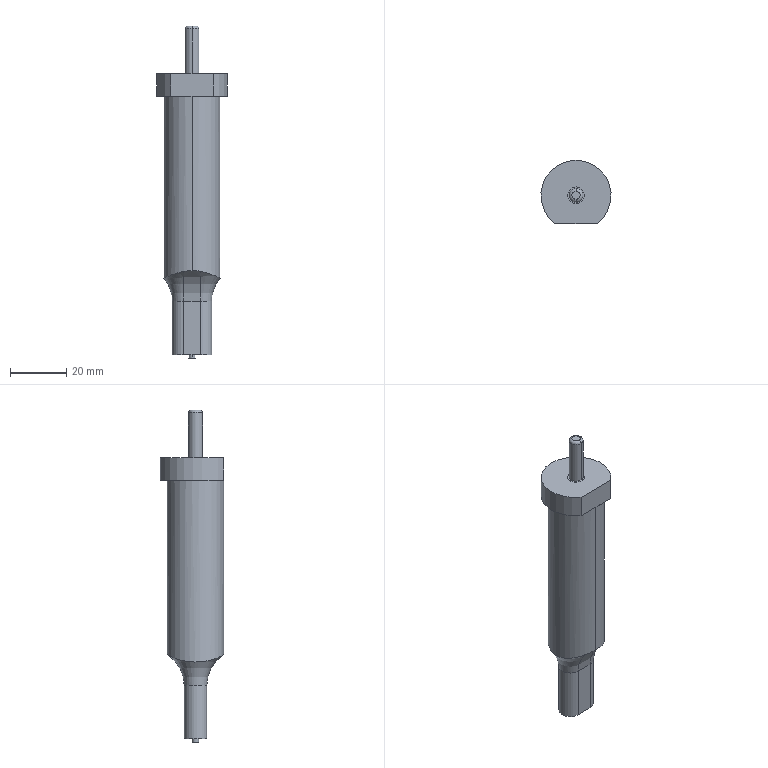Part | STEP file | 1_id3642_x_t | 1 solid | 27 faces | box 25 x 22.5 x 118.2 mm | volume 27347 mm3 | cylinder 14 | plane 9 | torus 4 | commonest cylinder face diameters 2.26 x2 5 x2 6 x2 8.05 x2 20 x2 25 x2
STEP:
#1=CARTESIAN_POINT('',(3587.234,-220.45,22.438));
#2=VERTEX_POINT('',#1);
#3=CARTESIAN_POINT('',(3587.234,-220.45,84.5));
#4=VERTEX_POINT('',#3);
#5=CARTESIAN_POINT('',(3587.234,-220.45,38.5));
#6=DIRECTION('',(0.,0.,1.));
#7=VECTOR('',#6,1.);
#8=LINE('',#5,#7);
#9=EDGE_CURVE('',#2,#4,#8,.T.);
#10=ORIENTED_EDGE('',*,*,#9,.F.);
#11=CARTESIAN_POINT('',(3584.234,-220.911,22.129));
#12=VERTEX_POINT('',#11);
#13=CARTESIAN_POINT('',(3587.234,-220.45,22.438));
#14=CARTESIAN_POINT('',(3586.2,-220.45,22.438));
#15=CARTESIAN_POINT('',(3585.2,-220.607,22.342));
#16=CARTESIAN_POINT('',(3584.234,-220.911,22.129));
#17=B_SPLINE_CURVE_WITH_KNOTS('',3,(#13,#14,#15,#16),.UNSPECIFIED.,.F.,.F.,(4,4),(0.,1.),.UNSPECIFIED.);
#18=EDGE_CURVE('',#2,#12,#17,.T.);
#19=ORIENTED_EDGE('',*,*,#18,.T.);
#20=CARTESIAN_POINT('',(3584.234,-239.989,22.129));
#21=VERTEX_POINT('',#20);
#22=CARTESIAN_POINT('',(3584.234,-220.911,22.129));
#23=CARTESIAN_POINT('',(3582.209,-221.547,21.68));
#24=CARTESIAN_POINT('',(3580.455,-222.805,21.143));
#25=CARTESIAN_POINT('',(3577.956,-226.171,20.175));
#26=CARTESIAN_POINT('',(3577.238,-228.29,19.779));
#27=CARTESIAN_POINT('',(3577.23,-232.57,19.774));
#28=CARTESIAN_POINT('',(3577.946,-234.707,20.17));
#29=CARTESIAN_POINT('',(3580.438,-238.079,21.137));
#30=CARTESIAN_POINT('',(3582.208,-239.352,21.68));
#31=CARTESIAN_POINT('',(3584.234,-239.989,22.129));
#32=B_SPLINE_CURVE_WITH_KNOTS('',3,(#22,#23,#24,#25,#26,#27,#28,#29,#30,#31),.UNSPECIFIED.,.F.,.F.,(4,2,2,2,4),(0.,0.25,0.5,0.75,1.),.UNSPECIFIED.);
#33=EDGE_CURVE('',#12,#21,#32,.T.);
#34=ORIENTED_EDGE('',*,*,#33,.T.);
#35=CARTESIAN_POINT('',(3587.234,-240.45,22.438));
#36=VERTEX_POINT('',#35);
#37=CARTESIAN_POINT('',(3584.234,-239.989,22.129));
#38=CARTESIAN_POINT('',(3585.2,-240.293,22.342));
#39=CARTESIAN_POINT('',(3586.2,-240.45,22.438));
#40=CARTESIAN_POINT('',(3587.234,-240.45,22.438));
#41=B_SPLINE_CURVE_WITH_KNOTS('',3,(#37,#38,#39,#40),.UNSPECIFIED.,.F.,.F.,(4,4),(0.,1.),.UNSPECIFIED.);
#42=EDGE_CURVE('',#21,#36,#41,.T.);
#43=ORIENTED_EDGE('',*,*,#42,.T.);
#44=CARTESIAN_POINT('',(3587.234,-240.45,84.5));
#45=VERTEX_POINT('',#44);
#46=CARTESIAN_POINT('',(3587.234,-240.45,38.5));
#47=DIRECTION('',(0.,0.,-1.));
#48=VECTOR('',#47,1.);
#49=LINE('',#46,#48);
#50=EDGE_CURVE('',#45,#36,#49,.T.);
#51=ORIENTED_EDGE('',*,*,#50,.F.);
#52=CARTESIAN_POINT('',(3587.234,-230.45,84.5));
#53=DIRECTION('',(0.,0.,1.));
#54=DIRECTION('',(0.,1.,0.));
#55=AXIS2_PLACEMENT_3D('',#52,#53,#54);
#56=CIRCLE('',#55,10.);
#57=EDGE_CURVE('',#4,#45,#56,.T.);
#58=ORIENTED_EDGE('',*,*,#57,.F.);
#59=EDGE_LOOP('',(#10,#19,#34,#43,#51,#58));
#60=FACE_OUTER_BOUND('',#59,.T.);
#61=CARTESIAN_POINT('',(3587.234,-230.45,38.5));
#62=DIRECTION('',(0.,0.,-1.));
#63=DIRECTION('',(0.,-1.,0.));
#64=AXIS2_PLACEMENT_3D('',#61,#62,#63);
#65=CYLINDRICAL_SURFACE('',#64,10.);
#66=ADVANCED_FACE('',(#60),#65,.T.);
#67=CARTESIAN_POINT('',(3587.234,-217.95,84.5));
#68=VERTEX_POINT('',#67);
#69=CARTESIAN_POINT('',(3587.234,-217.95,92.5));
#70=VERTEX_POINT('',#69);
#71=CARTESIAN_POINT('',(3587.234,-217.95,88.5));
#72=DIRECTION('',(0.,0.,1.));
#73=VECTOR('',#72,1.);
#74=LINE('',#71,#73);
#75=EDGE_CURVE('',#68,#70,#74,.T.);
#76=ORIENTED_EDGE('',*,*,#75,.F.);
#77=CARTESIAN_POINT('',(3579.734,-240.45,84.5));
#78=VERTEX_POINT('',#77);
#79=CARTESIAN_POINT('',(3587.234,-230.45,84.5));
#80=DIRECTION('',(0.,0.,1.));
#81=DIRECTION('',(0.,1.,0.));
#82=AXIS2_PLACEMENT_3D('',#79,#80,#81);
#83=CIRCLE('',#82,12.5);
#84=EDGE_CURVE('',#68,#78,#83,.T.);
#85=ORIENTED_EDGE('',*,*,#84,.T.);
#86=CARTESIAN_POINT('',(3579.734,-240.45,92.5));
#87=VERTEX_POINT('',#86);
#88=CARTESIAN_POINT('',(3579.734,-240.45,88.5));
#89=DIRECTION('',(0.,0.,1.));
#90=VECTOR('',#89,1.);
#91=LINE('',#88,#90);
#92=EDGE_CURVE('',#78,#87,#91,.T.);
#93=ORIENTED_EDGE('',*,*,#92,.T.);
#94=CARTESIAN_POINT('',(3587.234,-230.45,92.5));
#95=DIRECTION('',(0.,0.,1.));
#96=DIRECTION('',(0.,1.,0.));
#97=AXIS2_PLACEMENT_3D('',#94,#95,#96);
#98=CIRCLE('',#97,12.5);
#99=EDGE_CURVE('',#70,#87,#98,.T.);
#100=ORIENTED_EDGE('',*,*,#99,.F.);
#101=EDGE_LOOP('',(#76,#85,#93,#100));
#102=FACE_OUTER_BOUND('',#101,.T.);
#103=CARTESIAN_POINT('',(3587.234,-230.45,88.5));
#104=DIRECTION('',(0.,0.,-1.));
#105=DIRECTION('',(0.,-1.,0.));
#106=AXIS2_PLACEMENT_3D('',#103,#104,#105);
#107=CYLINDRICAL_SURFACE('',#106,12.5);
#108=ADVANCED_FACE('',(#102),#107,.T.);
#109=CARTESIAN_POINT('',(3587.234,-231.58,-7.5));
#110=VERTEX_POINT('',#109);
#111=CARTESIAN_POINT('',(3587.234,-231.58,-8.7));
#112=VERTEX_POINT('',#111);
#113=CARTESIAN_POINT('',(3587.234,-231.58,-7.5));
#114=DIRECTION('',(0.,0.,-1.));
#115=VECTOR('',#114,1.);
#116=LINE('',#113,#115);
#117=EDGE_CURVE('',#110,#112,#116,.T.);
#118=ORIENTED_EDGE('',*,*,#117,.F.);
#119=CARTESIAN_POINT('',(3587.234,-229.32,-7.5));
#120=VERTEX_POINT('',#119);
#121=CARTESIAN_POINT('',(3587.234,-230.45,-7.5));
#122=DIRECTION('',(0.,0.,1.));
#123=DIRECTION('',(0.,-1.,0.));
#124=AXIS2_PLACEMENT_3D('',#121,#122,#123);
#125=CIRCLE('',#124,1.13);
#126=EDGE_CURVE('',#120,#110,#125,.T.);
#127=ORIENTED_EDGE('',*,*,#126,.F.);
#128=CARTESIAN_POINT('',(3587.234,-229.32,-8.7));
#129=VERTEX_POINT('',#128);
#130=CARTESIAN_POINT('',(3587.234,-229.32,-7.5));
#131=DIRECTION('',(0.,0.,1.));
#132=VECTOR('',#131,1.);
#133=LINE('',#130,#132);
#134=EDGE_CURVE('',#129,#120,#133,.T.);
#135=ORIENTED_EDGE('',*,*,#134,.F.);
#136=CARTESIAN_POINT('',(3587.234,-230.45,-8.7));
#137=DIRECTION('',(0.,0.,1.));
#138=DIRECTION('',(0.,-1.,0.));
#139=AXIS2_PLACEMENT_3D('',#136,#137,#138);
#140=CIRCLE('',#139,1.13);
#141=EDGE_CURVE('',#129,#112,#140,.T.);
#142=ORIENTED_EDGE('',*,*,#141,.T.);
#143=EDGE_LOOP('',(#118,#127,#135,#142));
#144=FACE_OUTER_BOUND('',#143,.T.);
#145=CARTESIAN_POINT('',(3587.234,-230.45,-7.5));
#146=DIRECTION('',(0.,0.,1.));
#147=DIRECTION('',(0.,1.,0.));
#148=AXIS2_PLACEMENT_3D('',#145,#146,#147);
#149=CYLINDRICAL_SURFACE('',#148,1.13);
#150=ADVANCED_FACE('',(#144),#149,.T.);
#151=CARTESIAN_POINT('',(3587.234,-232.95,108.5));
#152=VERTEX_POINT('',#151);
#153=CARTESIAN_POINT('',(3587.234,-232.95,92.6));
#154=VERTEX_POINT('',#153);
#155=CARTESIAN_POINT('',(3587.234,-232.95,100.55));
#156=DIRECTION('',(0.,0.,-1.));
#157=VECTOR('',#156,1.);
#158=LINE('',#155,#157);
#159=EDGE_CURVE('',#152,#154,#158,.T.);
#160=ORIENTED_EDGE('',*,*,#159,.F.);
#161=CARTESIAN_POINT('',(3587.234,-227.95,108.5));
#162=VERTEX_POINT('',#161);
#163=CARTESIAN_POINT('',(3587.234,-230.45,108.5));
#164=DIRECTION('',(0.,0.,-1.));
#165=DIRECTION('',(0.,-1.,0.));
#166=AXIS2_PLACEMENT_3D('',#163,#164,#165);
#167=CIRCLE('',#166,2.5);
#168=EDGE_CURVE('',#152,#162,#167,.T.);
#169=ORIENTED_EDGE('',*,*,#168,.T.);
#170=CARTESIAN_POINT('',(3587.234,-227.95,92.6));
#171=VERTEX_POINT('',#170);
#172=CARTESIAN_POINT('',(3587.234,-227.95,100.55));
#173=DIRECTION('',(0.,0.,1.));
#174=VECTOR('',#173,1.);
#175=LINE('',#172,#174);
#176=EDGE_CURVE('',#171,#162,#175,.T.);
#177=ORIENTED_EDGE('',*,*,#176,.F.);
#178=CARTESIAN_POINT('',(3587.234,-230.45,92.6));
#179=DIRECTION('',(0.,0.,-1.));
#180=DIRECTION('',(0.,-1.,0.));
#181=AXIS2_PLACEMENT_3D('',#178,#179,#180);
#182=CIRCLE('',#181,2.5);
#183=EDGE_CURVE('',#154,#171,#182,.T.);
#184=ORIENTED_EDGE('',*,*,#183,.F.);
#185=EDGE_LOOP('',(#160,#169,#177,#184));
#186=FACE_OUTER_BOUND('',#185,.T.);
#187=CARTESIAN_POINT('',(3587.234,-230.45,100.55));
#188=DIRECTION('',(0.,0.,1.));
#189=DIRECTION('',(0.,1.,0.));
#190=AXIS2_PLACEMENT_3D('',#187,#188,#189);
#191=CYLINDRICAL_SURFACE('',#190,2.5);
#192=ADVANCED_FACE('',(#186),#191,.T.);
#193=CARTESIAN_POINT('',(3587.234,-228.95,109.5));
#194=VERTEX_POINT('',#193);
#195=CARTESIAN_POINT('',(3587.234,-228.95,108.5));
#196=DIRECTION('',(-1.,0.,0.));
#197=DIRECTION('',(0.,1.,0.));
#198=AXIS2_PLACEMENT_3D('',#195,#196,#197);
#199=CIRCLE('',#198,1.);
#200=EDGE_CURVE('',#194,#162,#199,.T.);
#201=ORIENTED_EDGE('',*,*,#200,.F.);
#202=CARTESIAN_POINT('',(3587.234,-231.95,109.5));
#203=VERTEX_POINT('',#202);
#204=CARTESIAN_POINT('',(3587.234,-230.45,109.5));
#205=DIRECTION('',(0.,0.,-1.));
#206=DIRECTION('',(0.,-1.,0.));
#207=AXIS2_PLACEMENT_3D('',#204,#205,#206);
#208=CIRCLE('',#207,1.5);
#209=EDGE_CURVE('',#194,#203,#208,.T.);
#210=ORIENTED_EDGE('',*,*,#209,.T.);
#211=CARTESIAN_POINT('',(3587.234,-231.95,108.5));
#212=DIRECTION('',(-1.,0.,0.));
#213=DIRECTION('',(0.,-1.,0.));
#214=AXIS2_PLACEMENT_3D('',#211,#212,#213);
#215=CIRCLE('',#214,1.);
#216=EDGE_CURVE('',#152,#203,#215,.T.);
#217=ORIENTED_EDGE('',*,*,#216,.F.);
#218=CARTESIAN_POINT('',(3587.234,-230.45,108.5));
#219=DIRECTION('',(0.,0.,-1.));
#220=DIRECTION('',(0.,-1.,0.));
#221=AXIS2_PLACEMENT_3D('',#218,#219,#220);
#222=CIRCLE('',#221,2.5);
#223=EDGE_CURVE('',#162,#152,#222,.T.);
#224=ORIENTED_EDGE('',*,*,#223,.F.);
#225=EDGE_LOOP('',(#201,#210,#217,#224));
#226=FACE_OUTER_BOUND('',#225,.T.);
#227=CARTESIAN_POINT('',(3587.234,-230.45,108.5));
#228=DIRECTION('',(0.,0.,-1.));
#229=DIRECTION('',(0.,-1.,0.));
#230=AXIS2_PLACEMENT_3D('',#227,#228,#229);
#231=TOROIDAL_SURFACE('',#230,1.5,1.);
#232=ADVANCED_FACE('',(#226),#231,.T.);
#233=CARTESIAN_POINT('',(3587.234,-233.45,92.6));
#234=VERTEX_POINT('',#233);
#235=CARTESIAN_POINT('',(3587.234,-233.45,92.5));
#236=VERTEX_POINT('',#235);
#237=CARTESIAN_POINT('',(3587.234,-233.45,92.55));
#238=DIRECTION('',(0.,0.,-1.));
#239=VECTOR('',#238,1.);
#240=LINE('',#237,#239);
#241=EDGE_CURVE('',#234,#236,#240,.T.);
#242=ORIENTED_EDGE('',*,*,#241,.F.);
#243=CARTESIAN_POINT('',(3587.234,-227.45,92.6));
#244=VERTEX_POINT('',#243);
#245=CARTESIAN_POINT('',(3587.234,-230.45,92.6));
#246=DIRECTION('',(0.,0.,-1.));
#247=DIRECTION('',(0.,-1.,0.));
#248=AXIS2_PLACEMENT_3D('',#245,#246,#247);
#249=CIRCLE('',#248,3.);
#250=EDGE_CURVE('',#234,#244,#249,.T.);
#251=ORIENTED_EDGE('',*,*,#250,.T.);
#252=CARTESIAN_POINT('',(3587.234,-227.45,92.5));
#253=VERTEX_POINT('',#252);
#254=CARTESIAN_POINT('',(3587.234,-227.45,92.55));
#255=DIRECTION('',(0.,0.,1.));
#256=VECTOR('',#255,1.);
#257=LINE('',#254,#256);
#258=EDGE_CURVE('',#253,#244,#257,.T.);
#259=ORIENTED_EDGE('',*,*,#258,.F.);
#260=CARTESIAN_POINT('',(3587.234,-230.45,92.5));
#261=DIRECTION('',(0.,0.,-1.));
#262=DIRECTION('',(0.,-1.,0.));
#263=AXIS2_PLACEMENT_3D('',#260,#261,#262);
#264=CIRCLE('',#263,3.);
#265=EDGE_CURVE('',#236,#253,#264,.T.);
#266=ORIENTED_EDGE('',*,*,#265,.F.);
#267=EDGE_LOOP('',(#242,#251,#259,#266));
#268=FACE_OUTER_BOUND('',#267,.T.);
#269=CARTESIAN_POINT('',(3587.234,-230.45,87.05));
#270=DIRECTION('',(0.,0.,1.));
#271=DIRECTION('',(0.,1.,0.));
#272=AXIS2_PLACEMENT_3D('',#269,#270,#271);
#273=CYLINDRICAL_SURFACE('',#272,3.);
#274=ADVANCED_FACE('',(#268),#273,.T.);
#275=ORIENTED_EDGE('',*,*,#241,.T.);
#276=CARTESIAN_POINT('',(3587.234,-230.45,92.5));
#277=DIRECTION('',(0.,0.,-1.));
#278=DIRECTION('',(0.,-1.,0.));
#279=AXIS2_PLACEMENT_3D('',#276,#277,#278);
#280=CIRCLE('',#279,3.);
#281=EDGE_CURVE('',#253,#236,#280,.T.);
#282=ORIENTED_EDGE('',*,*,#281,.F.);
#283=ORIENTED_EDGE('',*,*,#258,.T.);
#284=CARTESIAN_POINT('',(3587.234,-230.45,92.6));
#285=DIRECTION('',(0.,0.,-1.));
#286=DIRECTION('',(0.,-1.,0.));
#287=AXIS2_PLACEMENT_3D('',#284,#285,#286);
#288=CIRCLE('',#287,3.);
#289=EDGE_CURVE('',#244,#234,#288,.T.);
#290=ORIENTED_EDGE('',*,*,#289,.T.);
#291=EDGE_LOOP('',(#275,#282,#283,#290));
#292=FACE_OUTER_BOUND('',#291,.T.);
#293=CARTESIAN_POINT('',(3587.234,-230.45,87.05));
#294=DIRECTION('',(0.,0.,1.));
#295=DIRECTION('',(0.,1.,0.));
#296=AXIS2_PLACEMENT_3D('',#293,#294,#295);
#297=CYLINDRICAL_SURFACE('',#296,3.);
#298=ADVANCED_FACE('',(#292),#297,.T.);
#299=CARTESIAN_POINT('',(3587.234,-230.45,109.5));
#300=DIRECTION('',(0.,0.,-1.));
#301=DIRECTION('',(0.,-1.,0.));
#302=AXIS2_PLACEMENT_3D('',#299,#300,#301);
#303=CIRCLE('',#302,1.5);
#304=EDGE_CURVE('',#203,#194,#303,.T.);
#305=ORIENTED_EDGE('',*,*,#304,.F.);
#306=ORIENTED_EDGE('',*,*,#209,.F.);
#307=EDGE_LOOP('',(#305,#306));
#308=FACE_OUTER_BOUND('',#307,.T.);
#309=CARTESIAN_POINT('',(3587.234,-231.2,109.5));
#310=DIRECTION('',(0.,0.,1.));
#311=DIRECTION('',(0.,-1.,0.));
#312=AXIS2_PLACEMENT_3D('',#309,#310,#311);
#313=PLANE('',#312);
#314=ADVANCED_FACE('',(#308),#313,.T.);
#315=ORIENTED_EDGE('',*,*,#200,.T.);
#316=ORIENTED_EDGE('',*,*,#168,.F.);
#317=ORIENTED_EDGE('',*,*,#216,.T.);
#318=ORIENTED_EDGE('',*,*,#304,.T.);
#319=EDGE_LOOP('',(#315,#316,#317,#318));
#320=FACE_OUTER_BOUND('',#319,.T.);
#321=CARTESIAN_POINT('',(3587.234,-230.45,108.5));
#322=DIRECTION('',(0.,0.,-1.));
#323=DIRECTION('',(0.,-1.,0.));
#324=AXIS2_PLACEMENT_3D('',#321,#322,#323);
#325=TOROIDAL_SURFACE('',#324,1.5,1.);
#326=ADVANCED_FACE('',(#320),#325,.T.);
#327=ORIENTED_EDGE('',*,*,#159,.T.);
#328=CARTESIAN_POINT('',(3587.234,-230.45,92.6));
#329=DIRECTION('',(0.,0.,-1.));
#330=DIRECTION('',(0.,-1.,0.));
#331=AXIS2_PLACEMENT_3D('',#328,#329,#330);
#332=CIRCLE('',#331,2.5);
#333=EDGE_CURVE('',#171,#154,#332,.T.);
#334=ORIENTED_EDGE('',*,*,#333,.F.);
#335=ORIENTED_EDGE('',*,*,#176,.T.);
#336=ORIENTED_EDGE('',*,*,#223,.T.);
#337=EDGE_LOOP('',(#327,#334,#335,#336));
#338=FACE_OUTER_BOUND('',#337,.T.);
#339=CARTESIAN_POINT('',(3587.234,-230.45,100.55));
#340=DIRECTION('',(0.,0.,1.));
#341=DIRECTION('',(0.,1.,0.));
#342=AXIS2_PLACEMENT_3D('',#339,#340,#341);
#343=CYLINDRICAL_SURFACE('',#342,2.5);
#344=ADVANCED_FACE('',(#338),#343,.T.);
#345=ORIENTED_EDGE('',*,*,#250,.F.);
#346=ORIENTED_EDGE('',*,*,#289,.F.);
#347=EDGE_LOOP('',(#345,#346));
#348=FACE_BOUND('',#347,.T.);
#349=ORIENTED_EDGE('',*,*,#183,.T.);
#350=ORIENTED_EDGE('',*,*,#333,.T.);
#351=EDGE_LOOP('',(#349,#350));
#352=FACE_BOUND('',#351,.T.);
#353=CARTESIAN_POINT('',(3587.234,-233.2,92.6));
#354=DIRECTION('',(0.,0.,1.));
#355=DIRECTION('',(0.,-1.,0.));
#356=AXIS2_PLACEMENT_3D('',#353,#354,#355);
#357=PLANE('',#356);
#358=ADVANCED_FACE('',(#348,#352),#357,.T.);
#359=ORIENTED_EDGE('',*,*,#117,.T.);
#360=CARTESIAN_POINT('',(3587.234,-230.45,-8.7));
#361=DIRECTION('',(0.,0.,1.));
#362=DIRECTION('',(0.,-1.,0.));
#363=AXIS2_PLACEMENT_3D('',#360,#361,#362);
#364=CIRCLE('',#363,1.13);
#365=EDGE_CURVE('',#112,#129,#364,.T.);
#366=ORIENTED_EDGE('',*,*,#365,.T.);
#367=ORIENTED_EDGE('',*,*,#134,.T.);
#368=CARTESIAN_POINT('',(3587.234,-230.45,-7.5));
#369=DIRECTION('',(0.,0.,1.));
#370=DIRECTION('',(0.,-1.,0.));
#371=AXIS2_PLACEMENT_3D('',#368,#369,#370);
#372=CIRCLE('',#371,1.13);
#373=EDGE_CURVE('',#110,#120,#372,.T.);
#374=ORIENTED_EDGE('',*,*,#373,.F.);
#375=EDGE_LOOP('',(#359,#366,#367,#374));
#376=FACE_OUTER_BOUND('',#375,.T.);
#377=CARTESIAN_POINT('',(3587.234,-230.45,-7.5));
#378=DIRECTION('',(0.,0.,1.));
#379=DIRECTION('',(0.,1.,0.));
#380=AXIS2_PLACEMENT_3D('',#377,#378,#379);
#381=CYLINDRICAL_SURFACE('',#380,1.13);
#382=ADVANCED_FACE('',(#376),#381,.T.);
#383=ORIENTED_EDGE('',*,*,#365,.F.);
#384=ORIENTED_EDGE('',*,*,#141,.F.);
#385=EDGE_LOOP('',(#383,#384));
#386=FACE_OUTER_BOUND('',#385,.T.);
#387=CARTESIAN_POINT('',(3587.234,-230.45,-8.7));
#388=DIRECTION('',(0.,0.,1.));
#389=DIRECTION('',(0.,1.,0.));
#390=AXIS2_PLACEMENT_3D('',#387,#388,#389);
#391=PLANE('',#390);
#392=ADVANCED_FACE('',(#386),#391,.F.);
#393=CARTESIAN_POINT('',(3592.984,-240.45,84.5));
#394=DIRECTION('',(-1.,0.,0.));
#395=VECTOR('',#394,1.);
#396=LINE('',#393,#395);
#397=EDGE_CURVE('',#45,#78,#396,.T.);
#398=ORIENTED_EDGE('',*,*,#397,.F.);
#399=CARTESIAN_POINT('',(3594.734,-240.45,84.5));
#400=VERTEX_POINT('',#399);
#401=CARTESIAN_POINT('',(3592.984,-240.45,84.5));
#402=DIRECTION('',(-1.,0.,0.));
#403=VECTOR('',#402,1.);
#404=LINE('',#401,#403);
#405=EDGE_CURVE('',#400,#45,#404,.T.);
#406=ORIENTED_EDGE('',*,*,#405,.F.);
#407=CARTESIAN_POINT('',(3594.734,-240.45,92.5));
#408=VERTEX_POINT('',#407);
#409=CARTESIAN_POINT('',(3594.734,-240.45,88.5));
#410=DIRECTION('',(0.,0.,-1.));
#411=VECTOR('',#410,1.);
#412=LINE('',#409,#411);
#413=EDGE_CURVE('',#408,#400,#412,.T.);
#414=ORIENTED_EDGE('',*,*,#413,.F.);
#415=CARTESIAN_POINT('',(3592.984,-240.45,92.5));
#416=DIRECTION('',(1.,0.,0.));
#417=VECTOR('',#416,1.);
#418=LINE('',#415,#417);
#419=EDGE_CURVE('',#87,#408,#418,.T.);
#420=ORIENTED_EDGE('',*,*,#419,.F.);
#421=ORIENTED_EDGE('',*,*,#92,.F.);
#422=EDGE_LOOP('',(#398,#406,#414,#420,#421));
#423=FACE_OUTER_BOUND('',#422,.T.);
#424=CARTESIAN_POINT('',(3598.734,-240.45,92.51));
#425=DIRECTION('',(0.,1.,0.));
#426=DIRECTION('',(-1.,0.,0.));
#427=AXIS2_PLACEMENT_3D('',#424,#425,#426);
#428=PLANE('',#427);
#429=ADVANCED_FACE('',(#423),#428,.F.);
#430=ORIENTED_EDGE('',*,*,#75,.T.);
#431=CARTESIAN_POINT('',(3587.234,-230.45,92.5));
#432=DIRECTION('',(0.,0.,1.));
#433=DIRECTION('',(0.,1.,0.));
#434=AXIS2_PLACEMENT_3D('',#431,#432,#433);
#435=CIRCLE('',#434,12.5);
#436=EDGE_CURVE('',#408,#70,#435,.T.);
#437=ORIENTED_EDGE('',*,*,#436,.F.);
#438=ORIENTED_EDGE('',*,*,#413,.T.);
#439=CARTESIAN_POINT('',(3587.234,-230.45,84.5));
#440=DIRECTION('',(0.,0.,1.));
#441=DIRECTION('',(0.,1.,0.));
#442=AXIS2_PLACEMENT_3D('',#439,#440,#441);
#443=CIRCLE('',#442,12.5);
#444=EDGE_CURVE('',#400,#68,#443,.T.);
#445=ORIENTED_EDGE('',*,*,#444,.T.);
#446=EDGE_LOOP('',(#430,#437,#438,#445));
#447=FACE_OUTER_BOUND('',#446,.T.);
#448=CARTESIAN_POINT('',(3587.234,-230.45,88.5));
#449=DIRECTION('',(0.,0.,-1.));
#450=DIRECTION('',(0.,-1.,0.));
#451=AXIS2_PLACEMENT_3D('',#448,#449,#450);
#452=CYLINDRICAL_SURFACE('',#451,12.5);
#453=ADVANCED_FACE('',(#447),#452,.T.);
#454=ORIENTED_EDGE('',*,*,#405,.T.);
#455=CARTESIAN_POINT('',(3587.234,-230.45,84.5));
#456=DIRECTION('',(0.,0.,1.));
#457=DIRECTION('',(0.,1.,0.));
#458=AXIS2_PLACEMENT_3D('',#455,#456,#457);
#459=CIRCLE('',#458,10.);
#460=EDGE_CURVE('',#45,#4,#459,.T.);
#461=ORIENTED_EDGE('',*,*,#460,.T.);
#462=ORIENTED_EDGE('',*,*,#57,.T.);
#463=ORIENTED_EDGE('',*,*,#397,.T.);
#464=ORIENTED_EDGE('',*,*,#84,.F.);
#465=ORIENTED_EDGE('',*,*,#444,.F.);
#466=EDGE_LOOP('',(#454,#461,#462,#463,#464,#465));
#467=FACE_OUTER_BOUND('',#466,.T.);
#468=CARTESIAN_POINT('',(3587.234,-219.2,84.5));
#469=DIRECTION('',(0.,0.,-1.));
#470=DIRECTION('',(0.,1.,0.));
#471=AXIS2_PLACEMENT_3D('',#468,#469,#470);
#472=PLANE('',#471);
#473=ADVANCED_FACE('',(#467),#472,.T.);
#474=CARTESIAN_POINT('',(3584.234,-234.475,-7.5));
#475=VERTEX_POINT('',#474);
#476=CARTESIAN_POINT('',(3584.234,-226.425,-7.5));
#477=VERTEX_POINT('',#476);
#478=CARTESIAN_POINT('',(3584.234,-230.45,-7.5));
#479=DIRECTION('',(0.,0.,-1.));
#480=DIRECTION('',(0.,-1.,0.));
#481=AXIS2_PLACEMENT_3D('',#478,#479,#480);
#482=CIRCLE('',#481,4.025);
#483=EDGE_CURVE('',#475,#477,#482,.T.);
#484=ORIENTED_EDGE('',*,*,#483,.F.);
#485=CARTESIAN_POINT('',(3584.234,-234.475,11.5));
#486=VERTEX_POINT('',#485);
#487=CARTESIAN_POINT('',(3584.234,-234.475,2.));
#488=DIRECTION('',(0.,0.,1.));
#489=VECTOR('',#488,1.);
#490=LINE('',#487,#489);
#491=EDGE_CURVE('',#475,#486,#490,.T.);
#492=ORIENTED_EDGE('',*,*,#491,.T.);
#493=CARTESIAN_POINT('',(3584.234,-226.425,11.5));
#494=VERTEX_POINT('',#493);
#495=CARTESIAN_POINT('',(3584.234,-230.45,11.5));
#496=DIRECTION('',(0.,0.,-1.));
#497=DIRECTION('',(0.,-1.,0.));
#498=AXIS2_PLACEMENT_3D('',#495,#496,#497);
#499=CIRCLE('',#498,4.025);
#500=EDGE_CURVE('',#486,#494,#499,.T.);
#501=ORIENTED_EDGE('',*,*,#500,.T.);
#502=CARTESIAN_POINT('',(3584.234,-226.425,2.));
#503=DIRECTION('',(0.,0.,1.));
#504=VECTOR('',#503,1.);
#505=LINE('',#502,#504);
#506=EDGE_CURVE('',#477,#494,#505,.T.);
#507=ORIENTED_EDGE('',*,*,#506,.F.);
#508=EDGE_LOOP('',(#484,#492,#501,#507));
#509=FACE_OUTER_BOUND('',#508,.T.);
#510=CARTESIAN_POINT('',(3584.234,-230.45,1.5));
#511=DIRECTION('',(0.,0.,1.));
#512=DIRECTION('',(0.,1.,0.));
#513=AXIS2_PLACEMENT_3D('',#510,#511,#512);
#514=CYLINDRICAL_SURFACE('',#513,4.025);
#515=ADVANCED_FACE('',(#509),#514,.T.);
#516=ORIENTED_EDGE('',*,*,#33,.F.);
#517=CARTESIAN_POINT('',(3584.234,-213.425,11.5));
#518=DIRECTION('',(1.,0.,0.));
#519=DIRECTION('',(0.,1.,0.));
#520=AXIS2_PLACEMENT_3D('',#517,#518,#519);
#521=CIRCLE('',#520,13.);
#522=EDGE_CURVE('',#12,#494,#521,.T.);
#523=ORIENTED_EDGE('',*,*,#522,.T.);
#524=ORIENTED_EDGE('',*,*,#500,.F.);
#525=CARTESIAN_POINT('',(3584.234,-247.475,11.5));
#526=DIRECTION('',(-1.,0.,0.));
#527=DIRECTION('',(0.,-1.,0.));
#528=AXIS2_PLACEMENT_3D('',#525,#526,#527);
#529=CIRCLE('',#528,13.);
#530=EDGE_CURVE('',#21,#486,#529,.T.);
#531=ORIENTED_EDGE('',*,*,#530,.F.);
#532=EDGE_LOOP('',(#516,#523,#524,#531));
#533=FACE_OUTER_BOUND('',#532,.T.);
#534=CARTESIAN_POINT('',(3584.234,-230.45,11.5));
#535=DIRECTION('',(0.,0.,-1.));
#536=DIRECTION('',(0.,-1.,0.));
#537=AXIS2_PLACEMENT_3D('',#534,#535,#536);
#538=TOROIDAL_SURFACE('',#537,17.025,13.);
#539=ADVANCED_FACE('',(#533),#538,.F.);
#540=ORIENTED_EDGE('',*,*,#530,.T.);
#541=CARTESIAN_POINT('',(3590.234,-234.475,11.5));
#542=VERTEX_POINT('',#541);
#543=CARTESIAN_POINT('',(3607.234,-234.475,11.5));
#544=DIRECTION('',(-1.,0.,0.));
#545=VECTOR('',#544,1.);
#546=LINE('',#543,#545);
#547=EDGE_CURVE('',#542,#486,#546,.T.);
#548=ORIENTED_EDGE('',*,*,#547,.F.);
#549=CARTESIAN_POINT('',(3590.234,-239.989,22.129));
#550=VERTEX_POINT('',#549);
#551=CARTESIAN_POINT('',(3590.234,-247.475,11.5));
#552=DIRECTION('',(1.,0.,0.));
#553=DIRECTION('',(0.,-1.,0.));
#554=AXIS2_PLACEMENT_3D('',#551,#552,#553);
#555=CIRCLE('',#554,13.);
#556=EDGE_CURVE('',#542,#550,#555,.T.);
#557=ORIENTED_EDGE('',*,*,#556,.T.);
#558=CARTESIAN_POINT('',(3587.234,-240.45,22.438));
#559=CARTESIAN_POINT('',(3588.268,-240.45,22.438));
#560=CARTESIAN_POINT('',(3589.268,-240.293,22.342));
#561=CARTESIAN_POINT('',(3590.234,-239.989,22.129));
#562=B_SPLINE_CURVE_WITH_KNOTS('',3,(#558,#559,#560,#561),.UNSPECIFIED.,.F.,.F.,(4,4),(0.,1.),.UNSPECIFIED.);
#563=EDGE_CURVE('',#36,#550,#562,.T.);
#564=ORIENTED_EDGE('',*,*,#563,.F.);
#565=ORIENTED_EDGE('',*,*,#42,.F.);
#566=EDGE_LOOP('',(#540,#548,#557,#564,#565));
#567=FACE_OUTER_BOUND('',#566,.T.);
#568=CARTESIAN_POINT('',(3607.234,-247.475,11.5));
#569=DIRECTION('',(1.,0.,0.));
#570=DIRECTION('',(0.,-1.,0.));
#571=AXIS2_PLACEMENT_3D('',#568,#569,#570);
#572=CYLINDRICAL_SURFACE('',#571,13.);
#573=ADVANCED_FACE('',(#567),#572,.F.);
#574=ORIENTED_EDGE('',*,*,#491,.F.);
#575=CARTESIAN_POINT('',(3590.234,-234.475,-7.5));
#576=VERTEX_POINT('',#575);
#577=CARTESIAN_POINT('',(3597.234,-234.475,-7.5));
#578=DIRECTION('',(-1.,0.,0.));
#579=VECTOR('',#578,1.);
#580=LINE('',#577,#579);
#581=EDGE_CURVE('',#576,#475,#580,.T.);
#582=ORIENTED_EDGE('',*,*,#581,.F.);
#583=CARTESIAN_POINT('',(3590.234,-234.475,2.));
#584=DIRECTION('',(0.,0.,-1.));
#585=VECTOR('',#584,1.);
#586=LINE('',#583,#585);
#587=EDGE_CURVE('',#542,#576,#586,.T.);
#588=ORIENTED_EDGE('',*,*,#587,.F.);
#589=ORIENTED_EDGE('',*,*,#547,.T.);
#590=EDGE_LOOP('',(#574,#582,#588,#589));
#591=FACE_OUTER_BOUND('',#590,.T.);
#592=CARTESIAN_POINT('',(3607.234,-234.475,-8.5));
#593=DIRECTION('',(0.,1.,0.));
#594=DIRECTION('',(0.,0.,1.));
#595=AXIS2_PLACEMENT_3D('',#592,#593,#594);
#596=PLANE('',#595);
#597=ADVANCED_FACE('',(#591),#596,.F.);
#598=ORIENTED_EDGE('',*,*,#373,.T.);
#599=ORIENTED_EDGE('',*,*,#126,.T.);
#600=EDGE_LOOP('',(#598,#599));
#601=FACE_BOUND('',#600,.T.);
#602=ORIENTED_EDGE('',*,*,#483,.T.);
#603=CARTESIAN_POINT('',(3590.234,-226.425,-7.5));
#604=VERTEX_POINT('',#603);
#605=CARTESIAN_POINT('',(3597.234,-226.425,-7.5));
#606=DIRECTION('',(1.,0.,0.));
#607=VECTOR('',#606,1.);
#608=LINE('',#605,#607);
#609=EDGE_CURVE('',#477,#604,#608,.T.);
#610=ORIENTED_EDGE('',*,*,#609,.T.);
#611=CARTESIAN_POINT('',(3590.234,-230.45,-7.5));
#612=DIRECTION('',(0.,0.,-1.));
#613=DIRECTION('',(0.,-1.,0.));
#614=AXIS2_PLACEMENT_3D('',#611,#612,#613);
#615=CIRCLE('',#614,4.025);
#616=EDGE_CURVE('',#604,#576,#615,.T.);
#617=ORIENTED_EDGE('',*,*,#616,.T.);
#618=ORIENTED_EDGE('',*,*,#581,.T.);
#619=EDGE_LOOP('',(#602,#610,#617,#618));
#620=FACE_BOUND('',#619,.T.);
#621=CARTESIAN_POINT('',(3587.234,-225.45,-7.5));
#622=DIRECTION('',(0.,0.,-1.));
#623=DIRECTION('',(0.,1.,0.));
#624=AXIS2_PLACEMENT_3D('',#621,#622,#623);
#625=PLANE('',#624);
#626=ADVANCED_FACE('',(#601,#620),#625,.T.);
#627=CARTESIAN_POINT('',(3590.234,-220.911,22.129));
#628=VERTEX_POINT('',#627);
#629=CARTESIAN_POINT('',(3590.234,-239.989,22.129));
#630=CARTESIAN_POINT('',(3592.259,-239.353,21.68));
#631=CARTESIAN_POINT('',(3594.013,-238.095,21.143));
#632=CARTESIAN_POINT('',(3596.512,-234.729,20.175));
#633=CARTESIAN_POINT('',(3597.23,-232.61,19.779));
#634=CARTESIAN_POINT('',(3597.238,-228.33,19.774));
#635=CARTESIAN_POINT('',(3596.522,-226.193,20.17));
#636=CARTESIAN_POINT('',(3594.03,-222.821,21.137));
#637=CARTESIAN_POINT('',(3592.26,-221.548,21.68));
#638=CARTESIAN_POINT('',(3590.234,-220.911,22.129));
#639=B_SPLINE_CURVE_WITH_KNOTS('',3,(#629,#630,#631,#632,#633,#634,#635,#636,#637,#638),.UNSPECIFIED.,.F.,.F.,(4,2,2,2,4),(0.,0.25,0.5,0.75,1.),.UNSPECIFIED.);
#640=EDGE_CURVE('',#550,#628,#639,.T.);
#641=ORIENTED_EDGE('',*,*,#640,.F.);
#642=ORIENTED_EDGE('',*,*,#556,.F.);
#643=CARTESIAN_POINT('',(3590.234,-226.425,11.5));
#644=VERTEX_POINT('',#643);
#645=CARTESIAN_POINT('',(3590.234,-230.45,11.5));
#646=DIRECTION('',(0.,0.,1.));
#647=DIRECTION('',(0.,-1.,0.));
#648=AXIS2_PLACEMENT_3D('',#645,#646,#647);
#649=CIRCLE('',#648,4.025);
#650=EDGE_CURVE('',#542,#644,#649,.T.);
#651=ORIENTED_EDGE('',*,*,#650,.T.);
#652=CARTESIAN_POINT('',(3590.234,-213.425,11.5));
#653=DIRECTION('',(-1.,0.,0.));
#654=DIRECTION('',(0.,1.,0.));
#655=AXIS2_PLACEMENT_3D('',#652,#653,#654);
#656=CIRCLE('',#655,13.);
#657=EDGE_CURVE('',#644,#628,#656,.T.);
#658=ORIENTED_EDGE('',*,*,#657,.T.);
#659=EDGE_LOOP('',(#641,#642,#651,#658));
#660=FACE_OUTER_BOUND('',#659,.T.);
#661=CARTESIAN_POINT('',(3590.234,-230.45,11.5));
#662=DIRECTION('',(0.,0.,1.));
#663=DIRECTION('',(0.,1.,0.));
#664=AXIS2_PLACEMENT_3D('',#661,#662,#663);
#665=TOROIDAL_SURFACE('',#664,17.025,13.);
#666=ADVANCED_FACE('',(#660),#665,.F.);
#667=ORIENTED_EDGE('',*,*,#616,.F.);
#668=CARTESIAN_POINT('',(3590.234,-226.425,2.));
#669=DIRECTION('',(0.,0.,-1.));
#670=VECTOR('',#669,1.);
#671=LINE('',#668,#670);
#672=EDGE_CURVE('',#644,#604,#671,.T.);
#673=ORIENTED_EDGE('',*,*,#672,.F.);
#674=ORIENTED_EDGE('',*,*,#650,.F.);
#675=ORIENTED_EDGE('',*,*,#587,.T.);
#676=EDGE_LOOP('',(#667,#673,#674,#675));
#677=FACE_OUTER_BOUND('',#676,.T.);
#678=CARTESIAN_POINT('',(3590.234,-230.45,1.5));
#679=DIRECTION('',(0.,0.,-1.));
#680=DIRECTION('',(0.,1.,0.));
#681=AXIS2_PLACEMENT_3D('',#678,#679,#680);
#682=CYLINDRICAL_SURFACE('',#681,4.025);
#683=ADVANCED_FACE('',(#677),#682,.T.);
#684=ORIENTED_EDGE('',*,*,#9,.T.);
#685=ORIENTED_EDGE('',*,*,#460,.F.);
#686=ORIENTED_EDGE('',*,*,#50,.T.);
#687=ORIENTED_EDGE('',*,*,#563,.T.);
#688=ORIENTED_EDGE('',*,*,#640,.T.);
#689=CARTESIAN_POINT('',(3590.234,-220.911,22.129));
#690=CARTESIAN_POINT('',(3589.268,-220.607,22.342));
#691=CARTESIAN_POINT('',(3588.268,-220.45,22.438));
#692=CARTESIAN_POINT('',(3587.234,-220.45,22.438));
#693=B_SPLINE_CURVE_WITH_KNOTS('',3,(#689,#690,#691,#692),.UNSPECIFIED.,.F.,.F.,(4,4),(0.,1.),.UNSPECIFIED.);
#694=EDGE_CURVE('',#628,#2,#693,.T.);
#695=ORIENTED_EDGE('',*,*,#694,.T.);
#696=EDGE_LOOP('',(#684,#685,#686,#687,#688,#695));
#697=FACE_OUTER_BOUND('',#696,.T.);
#698=CARTESIAN_POINT('',(3587.234,-230.45,38.5));
#699=DIRECTION('',(0.,0.,-1.));
#700=DIRECTION('',(0.,-1.,0.));
#701=AXIS2_PLACEMENT_3D('',#698,#699,#700);
#702=CYLINDRICAL_SURFACE('',#701,10.);
#703=ADVANCED_FACE('',(#697),#702,.T.);
#704=ORIENTED_EDGE('',*,*,#522,.F.);
#705=ORIENTED_EDGE('',*,*,#18,.F.);
#706=ORIENTED_EDGE('',*,*,#694,.F.);
#707=ORIENTED_EDGE('',*,*,#657,.F.);
#708=CARTESIAN_POINT('',(3607.234,-226.425,11.5));
#709=DIRECTION('',(-1.,0.,0.));
#710=VECTOR('',#709,1.);
#711=LINE('',#708,#710);
#712=EDGE_CURVE('',#644,#494,#711,.T.);
#713=ORIENTED_EDGE('',*,*,#712,.T.);
#714=EDGE_LOOP('',(#704,#705,#706,#707,#713));
#715=FACE_OUTER_BOUND('',#714,.T.);
#716=CARTESIAN_POINT('',(3607.234,-213.425,11.5));
#717=DIRECTION('',(1.,0.,0.));
#718=DIRECTION('',(0.,0.,-1.));
#719=AXIS2_PLACEMENT_3D('',#716,#717,#718);
#720=CYLINDRICAL_SURFACE('',#719,13.);
#721=ADVANCED_FACE('',(#715),#720,.F.);
#722=ORIENTED_EDGE('',*,*,#506,.T.);
#723=ORIENTED_EDGE('',*,*,#712,.F.);
#724=ORIENTED_EDGE('',*,*,#672,.T.);
#725=ORIENTED_EDGE('',*,*,#609,.F.);
#726=EDGE_LOOP('',(#722,#723,#724,#725));
#727=FACE_OUTER_BOUND('',#726,.T.);
#728=CARTESIAN_POINT('',(3607.234,-226.425,11.5));
#729=DIRECTION('',(0.,-1.,0.));
#730=DIRECTION('',(0.,0.,-1.));
#731=AXIS2_PLACEMENT_3D('',#728,#729,#730);
#732=PLANE('',#731);
#733=ADVANCED_FACE('',(#727),#732,.F.);
#734=ORIENTED_EDGE('',*,*,#281,.T.);
#735=ORIENTED_EDGE('',*,*,#265,.T.);
#736=EDGE_LOOP('',(#734,#735));
#737=FACE_BOUND('',#736,.T.);
#738=ORIENTED_EDGE('',*,*,#419,.T.);
#739=ORIENTED_EDGE('',*,*,#436,.T.);
#740=ORIENTED_EDGE('',*,*,#99,.T.);
#741=EDGE_LOOP('',(#738,#739,#740));
#742=FACE_BOUND('',#741,.T.);
#743=CARTESIAN_POINT('',(3587.234,-224.2,92.5));
#744=DIRECTION('',(0.,0.,1.));
#745=DIRECTION('',(0.,-1.,0.));
#746=AXIS2_PLACEMENT_3D('',#743,#744,#745);
#747=PLANE('',#746);
#748=ADVANCED_FACE('',(#737,#742),#747,.T.);
#749=CLOSED_SHELL('',(#66,#108,#150,#192,#232,#274,#298,#314,#326,#344,#358,#382,#392,#429,#453,#473,#515,#539,#573,#597,#626,#666,#683,#703,#721,#733,#748));
#750=MANIFOLD_SOLID_BREP('',#749);
#751=(LENGTH_UNIT()NAMED_UNIT(*)SI_UNIT(.MILLI.,.METRE.));
#752=UNCERTAINTY_MEASURE_WITH_UNIT(LENGTH_MEASURE(0.0508),#751,'','');
#753=(NAMED_UNIT(*)PLANE_ANGLE_UNIT()SI_UNIT($,.RADIAN.));
#754=PLANE_ANGLE_MEASURE_WITH_UNIT(PLANE_ANGLE_MEASURE(0.01745),#753);
#755=DIMENSIONAL_EXPONENTS(0.,0.,0.,0.,0.,0.,0.);
#756=(CONVERSION_BASED_UNIT('DEGREE',#754)NAMED_UNIT(#755)PLANE_ANGLE_UNIT());
#757=(NAMED_UNIT(*)SI_UNIT($,.STERADIAN.)SOLID_ANGLE_UNIT());
#758=(GEOMETRIC_REPRESENTATION_CONTEXT(3)GLOBAL_UNCERTAINTY_ASSIGNED_CONTEXT((#752))GLOBAL_UNIT_ASSIGNED_CONTEXT((#751,#756,#757))REPRESENTATION_CONTEXT('',''));
#759=ADVANCED_BREP_SHAPE_REPRESENTATION('',(#750),#758);